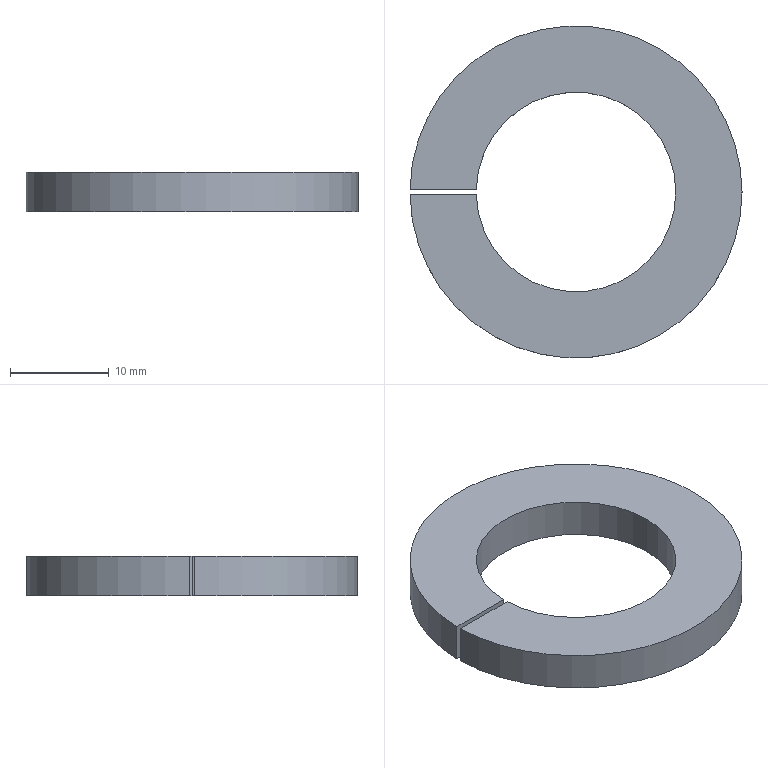Part | SolidWorks | features BaseBody 1 | 1 solid | 8 faces | box 33.598 x 33.6 x 4 mm | volume 2251 mm3 | cylinder 4 | plane 4 | commonest cylinder face diameters 20.2 x2 33.6 x2
STEP:
#1=CARTESIAN_POINT('',(10.1,0.,0.));
#2=VERTEX_POINT('',#1);
#3=CARTESIAN_POINT('',(-10.097,0.25,0.));
#4=VERTEX_POINT('',#3);
#5=CARTESIAN_POINT('',(0.,0.,0.));
#6=DIRECTION('',(0.,0.,1.));
#7=DIRECTION('',(1.,0.,0.));
#8=AXIS2_PLACEMENT_3D('',#5,#6,#7);
#9=CIRCLE('',#8,10.1);
#10=EDGE_CURVE('',#2,#4,#9,.T.);
#11=ORIENTED_EDGE('',*,*,#10,.F.);
#12=CARTESIAN_POINT('',(10.1,0.,4.));
#13=VERTEX_POINT('',#12);
#14=CARTESIAN_POINT('',(10.1,0.,4.));
#15=DIRECTION('',(0.,0.,1.));
#16=VECTOR('',#15,1000.);
#17=LINE('',#14,#16);
#18=EDGE_CURVE('',#2,#13,#17,.T.);
#19=ORIENTED_EDGE('',*,*,#18,.T.);
#20=CARTESIAN_POINT('',(-10.097,0.25,4.));
#21=VERTEX_POINT('',#20);
#22=CARTESIAN_POINT('',(0.,0.,4.));
#23=DIRECTION('',(0.,0.,-1.));
#24=DIRECTION('',(1.,0.,0.));
#25=AXIS2_PLACEMENT_3D('',#22,#23,#24);
#26=CIRCLE('',#25,10.1);
#27=EDGE_CURVE('',#21,#13,#26,.T.);
#28=ORIENTED_EDGE('',*,*,#27,.F.);
#29=CARTESIAN_POINT('',(-10.097,0.25,4.));
#30=DIRECTION('',(0.,0.,1.));
#31=VECTOR('',#30,1000.);
#32=LINE('',#29,#31);
#33=EDGE_CURVE('',#4,#21,#32,.T.);
#34=ORIENTED_EDGE('',*,*,#33,.F.);
#35=EDGE_LOOP('',(#11,#19,#28,#34));
#36=FACE_OUTER_BOUND('',#35,.T.);
#37=CARTESIAN_POINT('',(0.,0.,4.));
#38=DIRECTION('',(0.,0.,1.));
#39=DIRECTION('',(1.,0.,0.));
#40=AXIS2_PLACEMENT_3D('',#37,#38,#39);
#41=CYLINDRICAL_SURFACE('',#40,10.1);
#42=ADVANCED_FACE('',(#36),#41,.F.);
#43=CARTESIAN_POINT('',(-16.798,-0.25,0.));
#44=VERTEX_POINT('',#43);
#45=CARTESIAN_POINT('',(16.8,0.,0.));
#46=VERTEX_POINT('',#45);
#47=CARTESIAN_POINT('',(0.,0.,0.));
#48=DIRECTION('',(0.,0.,1.));
#49=DIRECTION('',(1.,0.,0.));
#50=AXIS2_PLACEMENT_3D('',#47,#48,#49);
#51=CIRCLE('',#50,16.8);
#52=EDGE_CURVE('',#44,#46,#51,.T.);
#53=ORIENTED_EDGE('',*,*,#52,.T.);
#54=CARTESIAN_POINT('',(16.8,0.,4.));
#55=VERTEX_POINT('',#54);
#56=CARTESIAN_POINT('',(16.8,0.,4.));
#57=DIRECTION('',(0.,0.,1.));
#58=VECTOR('',#57,1000.);
#59=LINE('',#56,#58);
#60=EDGE_CURVE('',#46,#55,#59,.T.);
#61=ORIENTED_EDGE('',*,*,#60,.T.);
#62=CARTESIAN_POINT('',(-16.798,-0.25,4.));
#63=VERTEX_POINT('',#62);
#64=CARTESIAN_POINT('',(0.,0.,4.));
#65=DIRECTION('',(0.,0.,1.));
#66=DIRECTION('',(1.,0.,0.));
#67=AXIS2_PLACEMENT_3D('',#64,#65,#66);
#68=CIRCLE('',#67,16.8);
#69=EDGE_CURVE('',#63,#55,#68,.T.);
#70=ORIENTED_EDGE('',*,*,#69,.F.);
#71=CARTESIAN_POINT('',(-16.798,-0.25,4.));
#72=DIRECTION('',(0.,0.,-1.));
#73=VECTOR('',#72,1000.);
#74=LINE('',#71,#73);
#75=EDGE_CURVE('',#63,#44,#74,.T.);
#76=ORIENTED_EDGE('',*,*,#75,.T.);
#77=EDGE_LOOP('',(#53,#61,#70,#76));
#78=FACE_OUTER_BOUND('',#77,.T.);
#79=CARTESIAN_POINT('',(0.,0.,4.));
#80=DIRECTION('',(0.,0.,1.));
#81=DIRECTION('',(1.,0.,0.));
#82=AXIS2_PLACEMENT_3D('',#79,#80,#81);
#83=CYLINDRICAL_SURFACE('',#82,16.8);
#84=ADVANCED_FACE('',(#78),#83,.T.);
#85=ORIENTED_EDGE('',*,*,#27,.T.);
#86=CARTESIAN_POINT('',(-10.097,-0.25,4.));
#87=VERTEX_POINT('',#86);
#88=CARTESIAN_POINT('',(0.,0.,4.));
#89=DIRECTION('',(0.,0.,-1.));
#90=DIRECTION('',(1.,0.,0.));
#91=AXIS2_PLACEMENT_3D('',#88,#89,#90);
#92=CIRCLE('',#91,10.1);
#93=EDGE_CURVE('',#13,#87,#92,.T.);
#94=ORIENTED_EDGE('',*,*,#93,.T.);
#95=CARTESIAN_POINT('',(0.,-0.25,4.));
#96=DIRECTION('',(-1.,0.,0.));
#97=VECTOR('',#96,1000.);
#98=LINE('',#95,#97);
#99=EDGE_CURVE('',#87,#63,#98,.T.);
#100=ORIENTED_EDGE('',*,*,#99,.T.);
#101=ORIENTED_EDGE('',*,*,#69,.T.);
#102=CARTESIAN_POINT('',(-16.798,0.25,4.));
#103=VERTEX_POINT('',#102);
#104=CARTESIAN_POINT('',(0.,0.,4.));
#105=DIRECTION('',(0.,0.,1.));
#106=DIRECTION('',(1.,0.,0.));
#107=AXIS2_PLACEMENT_3D('',#104,#105,#106);
#108=CIRCLE('',#107,16.8);
#109=EDGE_CURVE('',#55,#103,#108,.T.);
#110=ORIENTED_EDGE('',*,*,#109,.T.);
#111=CARTESIAN_POINT('',(0.,0.25,4.));
#112=DIRECTION('',(1.,0.,0.));
#113=VECTOR('',#112,1000.);
#114=LINE('',#111,#113);
#115=EDGE_CURVE('',#103,#21,#114,.T.);
#116=ORIENTED_EDGE('',*,*,#115,.T.);
#117=EDGE_LOOP('',(#85,#94,#100,#101,#110,#116));
#118=FACE_OUTER_BOUND('',#117,.T.);
#119=CARTESIAN_POINT('',(0.,0.,4.));
#120=DIRECTION('',(0.,0.,1.));
#121=DIRECTION('',(1.,0.,0.));
#122=AXIS2_PLACEMENT_3D('',#119,#120,#121);
#123=PLANE('',#122);
#124=ADVANCED_FACE('',(#118),#123,.T.);
#125=ORIENTED_EDGE('',*,*,#75,.F.);
#126=ORIENTED_EDGE('',*,*,#99,.F.);
#127=CARTESIAN_POINT('',(-10.097,-0.25,0.));
#128=VERTEX_POINT('',#127);
#129=CARTESIAN_POINT('',(-10.097,-0.25,4.));
#130=DIRECTION('',(0.,0.,1.));
#131=VECTOR('',#130,1000.);
#132=LINE('',#129,#131);
#133=EDGE_CURVE('',#128,#87,#132,.T.);
#134=ORIENTED_EDGE('',*,*,#133,.F.);
#135=CARTESIAN_POINT('',(-10.097,-0.25,0.));
#136=DIRECTION('',(1.,0.,0.));
#137=VECTOR('',#136,1000.);
#138=LINE('',#135,#137);
#139=EDGE_CURVE('',#44,#128,#138,.T.);
#140=ORIENTED_EDGE('',*,*,#139,.F.);
#141=EDGE_LOOP('',(#125,#126,#134,#140));
#142=FACE_OUTER_BOUND('',#141,.T.);
#143=CARTESIAN_POINT('',(-10.097,-0.25,4.));
#144=DIRECTION('',(0.,-1.,0.));
#145=DIRECTION('',(0.,0.,-1.));
#146=AXIS2_PLACEMENT_3D('',#143,#144,#145);
#147=PLANE('',#146);
#148=ADVANCED_FACE('',(#142),#147,.F.);
#149=ORIENTED_EDGE('',*,*,#18,.F.);
#150=CARTESIAN_POINT('',(0.,0.,0.));
#151=DIRECTION('',(0.,0.,1.));
#152=DIRECTION('',(1.,0.,0.));
#153=AXIS2_PLACEMENT_3D('',#150,#151,#152);
#154=CIRCLE('',#153,10.1);
#155=EDGE_CURVE('',#128,#2,#154,.T.);
#156=ORIENTED_EDGE('',*,*,#155,.F.);
#157=ORIENTED_EDGE('',*,*,#133,.T.);
#158=ORIENTED_EDGE('',*,*,#93,.F.);
#159=EDGE_LOOP('',(#149,#156,#157,#158));
#160=FACE_OUTER_BOUND('',#159,.T.);
#161=CARTESIAN_POINT('',(0.,0.,4.));
#162=DIRECTION('',(0.,0.,1.));
#163=DIRECTION('',(1.,0.,0.));
#164=AXIS2_PLACEMENT_3D('',#161,#162,#163);
#165=CYLINDRICAL_SURFACE('',#164,10.1);
#166=ADVANCED_FACE('',(#160),#165,.F.);
#167=ORIENTED_EDGE('',*,*,#33,.T.);
#168=ORIENTED_EDGE('',*,*,#115,.F.);
#169=CARTESIAN_POINT('',(-16.798,0.25,0.));
#170=VERTEX_POINT('',#169);
#171=CARTESIAN_POINT('',(-16.798,0.25,4.));
#172=DIRECTION('',(0.,0.,1.));
#173=VECTOR('',#172,1000.);
#174=LINE('',#171,#173);
#175=EDGE_CURVE('',#170,#103,#174,.T.);
#176=ORIENTED_EDGE('',*,*,#175,.F.);
#177=CARTESIAN_POINT('',(-16.798,0.25,0.));
#178=DIRECTION('',(-1.,0.,0.));
#179=VECTOR('',#178,1000.);
#180=LINE('',#177,#179);
#181=EDGE_CURVE('',#4,#170,#180,.T.);
#182=ORIENTED_EDGE('',*,*,#181,.F.);
#183=EDGE_LOOP('',(#167,#168,#176,#182));
#184=FACE_OUTER_BOUND('',#183,.T.);
#185=CARTESIAN_POINT('',(-16.798,0.25,4.));
#186=DIRECTION('',(0.,1.,0.));
#187=DIRECTION('',(0.,0.,1.));
#188=AXIS2_PLACEMENT_3D('',#185,#186,#187);
#189=PLANE('',#188);
#190=ADVANCED_FACE('',(#184),#189,.F.);
#191=ORIENTED_EDGE('',*,*,#60,.F.);
#192=CARTESIAN_POINT('',(0.,0.,0.));
#193=DIRECTION('',(0.,0.,1.));
#194=DIRECTION('',(1.,0.,0.));
#195=AXIS2_PLACEMENT_3D('',#192,#193,#194);
#196=CIRCLE('',#195,16.8);
#197=EDGE_CURVE('',#46,#170,#196,.T.);
#198=ORIENTED_EDGE('',*,*,#197,.T.);
#199=ORIENTED_EDGE('',*,*,#175,.T.);
#200=ORIENTED_EDGE('',*,*,#109,.F.);
#201=EDGE_LOOP('',(#191,#198,#199,#200));
#202=FACE_OUTER_BOUND('',#201,.T.);
#203=CARTESIAN_POINT('',(0.,0.,4.));
#204=DIRECTION('',(0.,0.,1.));
#205=DIRECTION('',(1.,0.,0.));
#206=AXIS2_PLACEMENT_3D('',#203,#204,#205);
#207=CYLINDRICAL_SURFACE('',#206,16.8);
#208=ADVANCED_FACE('',(#202),#207,.T.);
#209=ORIENTED_EDGE('',*,*,#139,.T.);
#210=ORIENTED_EDGE('',*,*,#155,.T.);
#211=ORIENTED_EDGE('',*,*,#10,.T.);
#212=ORIENTED_EDGE('',*,*,#181,.T.);
#213=ORIENTED_EDGE('',*,*,#197,.F.);
#214=ORIENTED_EDGE('',*,*,#52,.F.);
#215=EDGE_LOOP('',(#209,#210,#211,#212,#213,#214));
#216=FACE_OUTER_BOUND('',#215,.T.);
#217=CARTESIAN_POINT('',(0.,0.,0.));
#218=DIRECTION('',(0.,0.,1.));
#219=DIRECTION('',(1.,0.,0.));
#220=AXIS2_PLACEMENT_3D('',#217,#218,#219);
#221=PLANE('',#220);
#222=ADVANCED_FACE('',(#216),#221,.F.);
#223=CLOSED_SHELL('',(#42,#84,#124,#148,#166,#190,#208,#222));
#224=MANIFOLD_SOLID_BREP('',#223);
#225=CARTESIAN_POINT('',(0.,0.,0.));
#226=DIRECTION('',(0.,0.,1.));
#227=DIRECTION('',(1.,0.,0.));
#228=AXIS2_PLACEMENT_3D('',#225,#226,#227);
#229=(LENGTH_UNIT()NAMED_UNIT(*)SI_UNIT(.MILLI.,.METRE.));
#230=UNCERTAINTY_MEASURE_WITH_UNIT(LENGTH_MEASURE(0.00001),#229,'','');
#231=(NAMED_UNIT(*)PLANE_ANGLE_UNIT()SI_UNIT($,.RADIAN.));
#232=(NAMED_UNIT(*)SI_UNIT($,.STERADIAN.)SOLID_ANGLE_UNIT());
#233=(GEOMETRIC_REPRESENTATION_CONTEXT(3)GLOBAL_UNCERTAINTY_ASSIGNED_CONTEXT((#230))GLOBAL_UNIT_ASSIGNED_CONTEXT((#229,#231,#232))REPRESENTATION_CONTEXT('',''));
#234=ADVANCED_BREP_SHAPE_REPRESENTATION('',(#224,#228),#233);